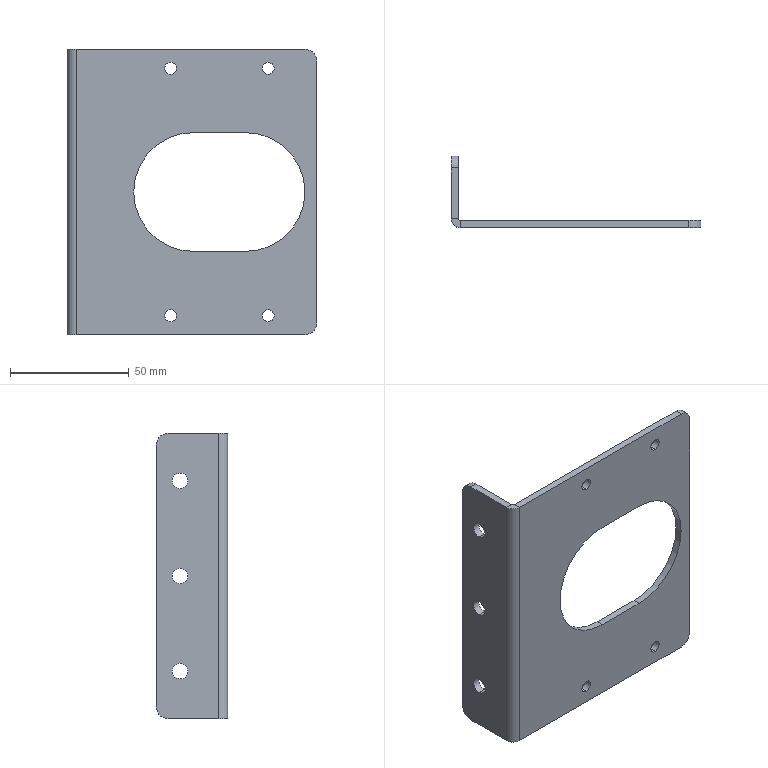Part | SolidWorks | features HoleWzd 2, BreakCorner 1, Cut 1, Extrusion 1, FlatPattern 1, ICE 1, SheetMetal 1, SolidToSheetMetal 1 | 1 solid | 36 faces | box 105 x 30 x 120 mm | volume 37376 mm3 | cylinder 22 | plane 14 | commonest cylinder face diameters 5 x8 6.6 x6 10 x4 50 x2 1.473 x1 7.473 x1
STEP:
#1=CARTESIAN_POINT('',(-52.5,5.,3.3));
#2=VERTEX_POINT('',#1);
#3=CARTESIAN_POINT('',(-52.5,5.,-3.3));
#4=VERTEX_POINT('',#3);
#5=CARTESIAN_POINT('',(-52.5,5.,0.));
#6=DIRECTION('',(1.,0.,0.));
#7=DIRECTION('',(0.,0.,-1.));
#8=AXIS2_PLACEMENT_3D('',#5,#6,#7);
#9=CIRCLE('',#8,3.3);
#10=EDGE_CURVE('',#2,#4,#9,.T.);
#11=ORIENTED_EDGE('',*,*,#10,.F.);
#12=CARTESIAN_POINT('',(-49.5,5.,3.3));
#13=VERTEX_POINT('',#12);
#14=CARTESIAN_POINT('',(-49.5,5.,3.3));
#15=DIRECTION('',(1.,0.,0.));
#16=VECTOR('',#15,1000.);
#17=LINE('',#14,#16);
#18=EDGE_CURVE('',#2,#13,#17,.T.);
#19=ORIENTED_EDGE('',*,*,#18,.T.);
#20=CARTESIAN_POINT('',(-49.5,5.,-3.3));
#21=VERTEX_POINT('',#20);
#22=CARTESIAN_POINT('',(-49.5,5.,0.));
#23=DIRECTION('',(1.,0.,0.));
#24=DIRECTION('',(0.,0.,-1.));
#25=AXIS2_PLACEMENT_3D('',#22,#23,#24);
#26=CIRCLE('',#25,3.3);
#27=EDGE_CURVE('',#13,#21,#26,.T.);
#28=ORIENTED_EDGE('',*,*,#27,.T.);
#29=CARTESIAN_POINT('',(-49.5,5.,-3.3));
#30=DIRECTION('',(1.,0.,0.));
#31=VECTOR('',#30,1000.);
#32=LINE('',#29,#31);
#33=EDGE_CURVE('',#4,#21,#32,.T.);
#34=ORIENTED_EDGE('',*,*,#33,.F.);
#35=EDGE_LOOP('',(#11,#19,#28,#34));
#36=FACE_OUTER_BOUND('',#35,.T.);
#37=CARTESIAN_POINT('',(-49.5,5.,0.));
#38=DIRECTION('',(1.,0.,0.));
#39=DIRECTION('',(0.,0.,-1.));
#40=AXIS2_PLACEMENT_3D('',#37,#38,#39);
#41=CYLINDRICAL_SURFACE('',#40,3.3);
#42=ADVANCED_FACE('',(#36),#41,.F.);
#43=CARTESIAN_POINT('',(-52.5,5.,43.3));
#44=VERTEX_POINT('',#43);
#45=CARTESIAN_POINT('',(-52.5,5.,36.7));
#46=VERTEX_POINT('',#45);
#47=CARTESIAN_POINT('',(-52.5,5.,40.));
#48=DIRECTION('',(1.,0.,0.));
#49=DIRECTION('',(0.,0.,-1.));
#50=AXIS2_PLACEMENT_3D('',#47,#48,#49);
#51=CIRCLE('',#50,3.3);
#52=EDGE_CURVE('',#44,#46,#51,.T.);
#53=ORIENTED_EDGE('',*,*,#52,.F.);
#54=CARTESIAN_POINT('',(-49.5,5.,43.3));
#55=VERTEX_POINT('',#54);
#56=CARTESIAN_POINT('',(-49.5,5.,43.3));
#57=DIRECTION('',(1.,0.,0.));
#58=VECTOR('',#57,1000.);
#59=LINE('',#56,#58);
#60=EDGE_CURVE('',#44,#55,#59,.T.);
#61=ORIENTED_EDGE('',*,*,#60,.T.);
#62=CARTESIAN_POINT('',(-49.5,5.,36.7));
#63=VERTEX_POINT('',#62);
#64=CARTESIAN_POINT('',(-49.5,5.,40.));
#65=DIRECTION('',(1.,0.,0.));
#66=DIRECTION('',(0.,0.,-1.));
#67=AXIS2_PLACEMENT_3D('',#64,#65,#66);
#68=CIRCLE('',#67,3.3);
#69=EDGE_CURVE('',#55,#63,#68,.T.);
#70=ORIENTED_EDGE('',*,*,#69,.T.);
#71=CARTESIAN_POINT('',(-49.5,5.,36.7));
#72=DIRECTION('',(1.,0.,0.));
#73=VECTOR('',#72,1000.);
#74=LINE('',#71,#73);
#75=EDGE_CURVE('',#46,#63,#74,.T.);
#76=ORIENTED_EDGE('',*,*,#75,.F.);
#77=EDGE_LOOP('',(#53,#61,#70,#76));
#78=FACE_OUTER_BOUND('',#77,.T.);
#79=CARTESIAN_POINT('',(-49.5,5.,40.));
#80=DIRECTION('',(1.,0.,0.));
#81=DIRECTION('',(0.,0.,-1.));
#82=AXIS2_PLACEMENT_3D('',#79,#80,#81);
#83=CYLINDRICAL_SURFACE('',#82,3.3);
#84=ADVANCED_FACE('',(#78),#83,.F.);
#85=CARTESIAN_POINT('',(-52.5,5.,-36.7));
#86=VERTEX_POINT('',#85);
#87=CARTESIAN_POINT('',(-52.5,5.,-43.3));
#88=VERTEX_POINT('',#87);
#89=CARTESIAN_POINT('',(-52.5,5.,-40.));
#90=DIRECTION('',(1.,0.,0.));
#91=DIRECTION('',(0.,0.,-1.));
#92=AXIS2_PLACEMENT_3D('',#89,#90,#91);
#93=CIRCLE('',#92,3.3);
#94=EDGE_CURVE('',#86,#88,#93,.T.);
#95=ORIENTED_EDGE('',*,*,#94,.F.);
#96=CARTESIAN_POINT('',(-49.5,5.,-36.7));
#97=VERTEX_POINT('',#96);
#98=CARTESIAN_POINT('',(-49.5,5.,-36.7));
#99=DIRECTION('',(1.,0.,0.));
#100=VECTOR('',#99,1000.);
#101=LINE('',#98,#100);
#102=EDGE_CURVE('',#86,#97,#101,.T.);
#103=ORIENTED_EDGE('',*,*,#102,.T.);
#104=CARTESIAN_POINT('',(-49.5,5.,-43.3));
#105=VERTEX_POINT('',#104);
#106=CARTESIAN_POINT('',(-49.5,5.,-40.));
#107=DIRECTION('',(1.,0.,0.));
#108=DIRECTION('',(0.,0.,-1.));
#109=AXIS2_PLACEMENT_3D('',#106,#107,#108);
#110=CIRCLE('',#109,3.3);
#111=EDGE_CURVE('',#97,#105,#110,.T.);
#112=ORIENTED_EDGE('',*,*,#111,.T.);
#113=CARTESIAN_POINT('',(-49.5,5.,-43.3));
#114=DIRECTION('',(1.,0.,0.));
#115=VECTOR('',#114,1000.);
#116=LINE('',#113,#115);
#117=EDGE_CURVE('',#88,#105,#116,.T.);
#118=ORIENTED_EDGE('',*,*,#117,.F.);
#119=EDGE_LOOP('',(#95,#103,#112,#118));
#120=FACE_OUTER_BOUND('',#119,.T.);
#121=CARTESIAN_POINT('',(-49.5,5.,-40.));
#122=DIRECTION('',(1.,0.,0.));
#123=DIRECTION('',(0.,0.,-1.));
#124=AXIS2_PLACEMENT_3D('',#121,#122,#123);
#125=CYLINDRICAL_SURFACE('',#124,3.3);
#126=ADVANCED_FACE('',(#120),#125,.F.);
#127=CARTESIAN_POINT('',(-9.,-15.,-54.5));
#128=VERTEX_POINT('',#127);
#129=CARTESIAN_POINT('',(-9.,-15.,-49.5));
#130=VERTEX_POINT('',#129);
#131=CARTESIAN_POINT('',(-9.,-15.,-52.));
#132=DIRECTION('',(0.,1.,0.));
#133=DIRECTION('',(0.,0.,1.));
#134=AXIS2_PLACEMENT_3D('',#131,#132,#133);
#135=CIRCLE('',#134,2.5);
#136=EDGE_CURVE('',#128,#130,#135,.T.);
#137=ORIENTED_EDGE('',*,*,#136,.F.);
#138=CARTESIAN_POINT('',(-9.,-12.,-54.5));
#139=VERTEX_POINT('',#138);
#140=CARTESIAN_POINT('',(-9.,-12.,-54.5));
#141=DIRECTION('',(0.,1.,0.));
#142=VECTOR('',#141,1000.);
#143=LINE('',#140,#142);
#144=EDGE_CURVE('',#128,#139,#143,.T.);
#145=ORIENTED_EDGE('',*,*,#144,.T.);
#146=CARTESIAN_POINT('',(-9.,-12.,-49.5));
#147=VERTEX_POINT('',#146);
#148=CARTESIAN_POINT('',(-9.,-12.,-52.));
#149=DIRECTION('',(0.,1.,0.));
#150=DIRECTION('',(0.,0.,1.));
#151=AXIS2_PLACEMENT_3D('',#148,#149,#150);
#152=CIRCLE('',#151,2.5);
#153=EDGE_CURVE('',#139,#147,#152,.T.);
#154=ORIENTED_EDGE('',*,*,#153,.T.);
#155=CARTESIAN_POINT('',(-9.,-12.,-49.5));
#156=DIRECTION('',(0.,1.,0.));
#157=VECTOR('',#156,1000.);
#158=LINE('',#155,#157);
#159=EDGE_CURVE('',#130,#147,#158,.T.);
#160=ORIENTED_EDGE('',*,*,#159,.F.);
#161=EDGE_LOOP('',(#137,#145,#154,#160));
#162=FACE_OUTER_BOUND('',#161,.T.);
#163=CARTESIAN_POINT('',(-9.,-12.,-52.));
#164=DIRECTION('',(0.,1.,0.));
#165=DIRECTION('',(0.,0.,1.));
#166=AXIS2_PLACEMENT_3D('',#163,#164,#165);
#167=CYLINDRICAL_SURFACE('',#166,2.5);
#168=ADVANCED_FACE('',(#162),#167,.F.);
#169=CARTESIAN_POINT('',(32.,-15.,-54.5));
#170=VERTEX_POINT('',#169);
#171=CARTESIAN_POINT('',(32.,-15.,-49.5));
#172=VERTEX_POINT('',#171);
#173=CARTESIAN_POINT('',(32.,-15.,-52.));
#174=DIRECTION('',(0.,1.,0.));
#175=DIRECTION('',(0.,0.,1.));
#176=AXIS2_PLACEMENT_3D('',#173,#174,#175);
#177=CIRCLE('',#176,2.5);
#178=EDGE_CURVE('',#170,#172,#177,.T.);
#179=ORIENTED_EDGE('',*,*,#178,.F.);
#180=CARTESIAN_POINT('',(32.,-12.,-54.5));
#181=VERTEX_POINT('',#180);
#182=CARTESIAN_POINT('',(32.,-12.,-54.5));
#183=DIRECTION('',(0.,1.,0.));
#184=VECTOR('',#183,1000.);
#185=LINE('',#182,#184);
#186=EDGE_CURVE('',#170,#181,#185,.T.);
#187=ORIENTED_EDGE('',*,*,#186,.T.);
#188=CARTESIAN_POINT('',(32.,-12.,-49.5));
#189=VERTEX_POINT('',#188);
#190=CARTESIAN_POINT('',(32.,-12.,-52.));
#191=DIRECTION('',(0.,1.,0.));
#192=DIRECTION('',(0.,0.,1.));
#193=AXIS2_PLACEMENT_3D('',#190,#191,#192);
#194=CIRCLE('',#193,2.5);
#195=EDGE_CURVE('',#181,#189,#194,.T.);
#196=ORIENTED_EDGE('',*,*,#195,.T.);
#197=CARTESIAN_POINT('',(32.,-12.,-49.5));
#198=DIRECTION('',(0.,1.,0.));
#199=VECTOR('',#198,1000.);
#200=LINE('',#197,#199);
#201=EDGE_CURVE('',#172,#189,#200,.T.);
#202=ORIENTED_EDGE('',*,*,#201,.F.);
#203=EDGE_LOOP('',(#179,#187,#196,#202));
#204=FACE_OUTER_BOUND('',#203,.T.);
#205=CARTESIAN_POINT('',(32.,-12.,-52.));
#206=DIRECTION('',(0.,1.,0.));
#207=DIRECTION('',(0.,0.,1.));
#208=AXIS2_PLACEMENT_3D('',#205,#206,#207);
#209=CYLINDRICAL_SURFACE('',#208,2.5);
#210=ADVANCED_FACE('',(#204),#209,.F.);
#211=CARTESIAN_POINT('',(32.,-15.,49.5));
#212=VERTEX_POINT('',#211);
#213=CARTESIAN_POINT('',(32.,-15.,54.5));
#214=VERTEX_POINT('',#213);
#215=CARTESIAN_POINT('',(32.,-15.,52.));
#216=DIRECTION('',(0.,1.,0.));
#217=DIRECTION('',(0.,0.,1.));
#218=AXIS2_PLACEMENT_3D('',#215,#216,#217);
#219=CIRCLE('',#218,2.5);
#220=EDGE_CURVE('',#212,#214,#219,.T.);
#221=ORIENTED_EDGE('',*,*,#220,.F.);
#222=CARTESIAN_POINT('',(32.,-12.,49.5));
#223=VERTEX_POINT('',#222);
#224=CARTESIAN_POINT('',(32.,-12.,49.5));
#225=DIRECTION('',(0.,1.,0.));
#226=VECTOR('',#225,1000.);
#227=LINE('',#224,#226);
#228=EDGE_CURVE('',#212,#223,#227,.T.);
#229=ORIENTED_EDGE('',*,*,#228,.T.);
#230=CARTESIAN_POINT('',(32.,-12.,54.5));
#231=VERTEX_POINT('',#230);
#232=CARTESIAN_POINT('',(32.,-12.,52.));
#233=DIRECTION('',(0.,1.,0.));
#234=DIRECTION('',(0.,0.,1.));
#235=AXIS2_PLACEMENT_3D('',#232,#233,#234);
#236=CIRCLE('',#235,2.5);
#237=EDGE_CURVE('',#223,#231,#236,.T.);
#238=ORIENTED_EDGE('',*,*,#237,.T.);
#239=CARTESIAN_POINT('',(32.,-12.,54.5));
#240=DIRECTION('',(0.,1.,0.));
#241=VECTOR('',#240,1000.);
#242=LINE('',#239,#241);
#243=EDGE_CURVE('',#214,#231,#242,.T.);
#244=ORIENTED_EDGE('',*,*,#243,.F.);
#245=EDGE_LOOP('',(#221,#229,#238,#244));
#246=FACE_OUTER_BOUND('',#245,.T.);
#247=CARTESIAN_POINT('',(32.,-12.,52.));
#248=DIRECTION('',(0.,1.,0.));
#249=DIRECTION('',(0.,0.,1.));
#250=AXIS2_PLACEMENT_3D('',#247,#248,#249);
#251=CYLINDRICAL_SURFACE('',#250,2.5);
#252=ADVANCED_FACE('',(#246),#251,.F.);
#253=CARTESIAN_POINT('',(-9.,-15.,49.5));
#254=VERTEX_POINT('',#253);
#255=CARTESIAN_POINT('',(-9.,-15.,54.5));
#256=VERTEX_POINT('',#255);
#257=CARTESIAN_POINT('',(-9.,-15.,52.));
#258=DIRECTION('',(0.,1.,0.));
#259=DIRECTION('',(0.,0.,1.));
#260=AXIS2_PLACEMENT_3D('',#257,#258,#259);
#261=CIRCLE('',#260,2.5);
#262=EDGE_CURVE('',#254,#256,#261,.T.);
#263=ORIENTED_EDGE('',*,*,#262,.F.);
#264=CARTESIAN_POINT('',(-9.,-12.,49.5));
#265=VERTEX_POINT('',#264);
#266=CARTESIAN_POINT('',(-9.,-12.,49.5));
#267=DIRECTION('',(0.,1.,0.));
#268=VECTOR('',#267,1000.);
#269=LINE('',#266,#268);
#270=EDGE_CURVE('',#254,#265,#269,.T.);
#271=ORIENTED_EDGE('',*,*,#270,.T.);
#272=CARTESIAN_POINT('',(-9.,-12.,54.5));
#273=VERTEX_POINT('',#272);
#274=CARTESIAN_POINT('',(-9.,-12.,52.));
#275=DIRECTION('',(0.,1.,0.));
#276=DIRECTION('',(0.,0.,1.));
#277=AXIS2_PLACEMENT_3D('',#274,#275,#276);
#278=CIRCLE('',#277,2.5);
#279=EDGE_CURVE('',#265,#273,#278,.T.);
#280=ORIENTED_EDGE('',*,*,#279,.T.);
#281=CARTESIAN_POINT('',(-9.,-12.,54.5));
#282=DIRECTION('',(0.,1.,0.));
#283=VECTOR('',#282,1000.);
#284=LINE('',#281,#283);
#285=EDGE_CURVE('',#256,#273,#284,.T.);
#286=ORIENTED_EDGE('',*,*,#285,.F.);
#287=EDGE_LOOP('',(#263,#271,#280,#286));
#288=FACE_OUTER_BOUND('',#287,.T.);
#289=CARTESIAN_POINT('',(-9.,-12.,52.));
#290=DIRECTION('',(0.,1.,0.));
#291=DIRECTION('',(0.,0.,1.));
#292=AXIS2_PLACEMENT_3D('',#289,#290,#291);
#293=CYLINDRICAL_SURFACE('',#292,2.5);
#294=ADVANCED_FACE('',(#288),#293,.F.);
#295=CARTESIAN_POINT('',(-48.763,-12.,-60.));
#296=VERTEX_POINT('',#295);
#297=CARTESIAN_POINT('',(47.5,-12.,-60.));
#298=VERTEX_POINT('',#297);
#299=CARTESIAN_POINT('',(-52.5,-12.,-60.));
#300=DIRECTION('',(1.,0.,0.));
#301=VECTOR('',#300,1000.);
#302=LINE('',#299,#301);
#303=EDGE_CURVE('',#296,#298,#302,.T.);
#304=ORIENTED_EDGE('',*,*,#303,.T.);
#305=CARTESIAN_POINT('',(47.5,-15.,-60.));
#306=VERTEX_POINT('',#305);
#307=CARTESIAN_POINT('',(47.5,-15.,-60.));
#308=DIRECTION('',(0.,-1.,0.));
#309=VECTOR('',#308,1000.);
#310=LINE('',#307,#309);
#311=EDGE_CURVE('',#298,#306,#310,.T.);
#312=ORIENTED_EDGE('',*,*,#311,.T.);
#313=CARTESIAN_POINT('',(-48.763,-15.,-60.));
#314=VERTEX_POINT('',#313);
#315=CARTESIAN_POINT('',(-52.5,-15.,-60.));
#316=DIRECTION('',(1.,0.,0.));
#317=VECTOR('',#316,1000.);
#318=LINE('',#315,#317);
#319=EDGE_CURVE('',#314,#306,#318,.T.);
#320=ORIENTED_EDGE('',*,*,#319,.F.);
#321=CARTESIAN_POINT('',(-48.763,-15.,-60.));
#322=DIRECTION('',(0.,-1.,0.));
#323=VECTOR('',#322,1000.);
#324=LINE('',#321,#323);
#325=EDGE_CURVE('',#296,#314,#324,.T.);
#326=ORIENTED_EDGE('',*,*,#325,.F.);
#327=EDGE_LOOP('',(#304,#312,#320,#326));
#328=FACE_OUTER_BOUND('',#327,.T.);
#329=CARTESIAN_POINT('',(-52.5,-15.,-60.));
#330=DIRECTION('',(0.,0.,1.));
#331=DIRECTION('',(1.,0.,0.));
#332=AXIS2_PLACEMENT_3D('',#329,#330,#331);
#333=PLANE('',#332);
#334=ADVANCED_FACE('',(#328),#333,.F.);
#335=CARTESIAN_POINT('',(52.5,-15.,55.));
#336=VERTEX_POINT('',#335);
#337=CARTESIAN_POINT('',(52.5,-15.,-55.));
#338=VERTEX_POINT('',#337);
#339=CARTESIAN_POINT('',(52.5,-15.,60.));
#340=DIRECTION('',(0.,0.,-1.));
#341=VECTOR('',#340,1000.);
#342=LINE('',#339,#341);
#343=EDGE_CURVE('',#336,#338,#342,.T.);
#344=ORIENTED_EDGE('',*,*,#343,.T.);
#345=CARTESIAN_POINT('',(52.5,-12.,-55.));
#346=VERTEX_POINT('',#345);
#347=CARTESIAN_POINT('',(52.5,-15.,-55.));
#348=DIRECTION('',(0.,1.,0.));
#349=VECTOR('',#348,1000.);
#350=LINE('',#347,#349);
#351=EDGE_CURVE('',#338,#346,#350,.T.);
#352=ORIENTED_EDGE('',*,*,#351,.T.);
#353=CARTESIAN_POINT('',(52.5,-12.,55.));
#354=VERTEX_POINT('',#353);
#355=CARTESIAN_POINT('',(52.5,-12.,60.));
#356=DIRECTION('',(0.,0.,-1.));
#357=VECTOR('',#356,1000.);
#358=LINE('',#355,#357);
#359=EDGE_CURVE('',#354,#346,#358,.T.);
#360=ORIENTED_EDGE('',*,*,#359,.F.);
#361=CARTESIAN_POINT('',(52.5,-15.,55.));
#362=DIRECTION('',(0.,-1.,0.));
#363=VECTOR('',#362,1000.);
#364=LINE('',#361,#363);
#365=EDGE_CURVE('',#354,#336,#364,.T.);
#366=ORIENTED_EDGE('',*,*,#365,.T.);
#367=EDGE_LOOP('',(#344,#352,#360,#366));
#368=FACE_OUTER_BOUND('',#367,.T.);
#369=CARTESIAN_POINT('',(52.5,-15.,60.));
#370=DIRECTION('',(1.,0.,0.));
#371=DIRECTION('',(0.,0.,-1.));
#372=AXIS2_PLACEMENT_3D('',#369,#370,#371);
#373=PLANE('',#372);
#374=ADVANCED_FACE('',(#368),#373,.T.);
#375=CARTESIAN_POINT('',(-48.763,-15.,60.));
#376=VERTEX_POINT('',#375);
#377=CARTESIAN_POINT('',(47.5,-15.,60.));
#378=VERTEX_POINT('',#377);
#379=CARTESIAN_POINT('',(-52.5,-15.,60.));
#380=DIRECTION('',(1.,0.,0.));
#381=VECTOR('',#380,1000.);
#382=LINE('',#379,#381);
#383=EDGE_CURVE('',#376,#378,#382,.T.);
#384=ORIENTED_EDGE('',*,*,#383,.T.);
#385=CARTESIAN_POINT('',(47.5,-12.,60.));
#386=VERTEX_POINT('',#385);
#387=CARTESIAN_POINT('',(47.5,-15.,60.));
#388=DIRECTION('',(0.,1.,0.));
#389=VECTOR('',#388,1000.);
#390=LINE('',#387,#389);
#391=EDGE_CURVE('',#378,#386,#390,.T.);
#392=ORIENTED_EDGE('',*,*,#391,.T.);
#393=CARTESIAN_POINT('',(-48.763,-12.,60.));
#394=VERTEX_POINT('',#393);
#395=CARTESIAN_POINT('',(-52.5,-12.,60.));
#396=DIRECTION('',(1.,0.,0.));
#397=VECTOR('',#396,1000.);
#398=LINE('',#395,#397);
#399=EDGE_CURVE('',#394,#386,#398,.T.);
#400=ORIENTED_EDGE('',*,*,#399,.F.);
#401=CARTESIAN_POINT('',(-48.763,-15.,60.));
#402=DIRECTION('',(0.,-1.,0.));
#403=VECTOR('',#402,1000.);
#404=LINE('',#401,#403);
#405=EDGE_CURVE('',#394,#376,#404,.T.);
#406=ORIENTED_EDGE('',*,*,#405,.T.);
#407=EDGE_LOOP('',(#384,#392,#400,#406));
#408=FACE_OUTER_BOUND('',#407,.T.);
#409=CARTESIAN_POINT('',(-52.5,-15.,60.));
#410=DIRECTION('',(0.,0.,1.));
#411=DIRECTION('',(1.,0.,0.));
#412=AXIS2_PLACEMENT_3D('',#409,#410,#411);
#413=PLANE('',#412);
#414=ADVANCED_FACE('',(#408),#413,.T.);
#415=ORIENTED_EDGE('',*,*,#405,.F.);
#416=CARTESIAN_POINT('',(-49.5,-11.263,60.));
#417=VERTEX_POINT('',#416);
#418=CARTESIAN_POINT('',(-48.763,-11.263,60.));
#419=DIRECTION('',(0.,0.,-1.));
#420=DIRECTION('',(-1.,0.,0.));
#421=AXIS2_PLACEMENT_3D('',#418,#419,#420);
#422=CIRCLE('',#421,0.7366);
#423=EDGE_CURVE('',#394,#417,#422,.T.);
#424=ORIENTED_EDGE('',*,*,#423,.T.);
#425=CARTESIAN_POINT('',(-52.5,-11.263,60.));
#426=VERTEX_POINT('',#425);
#427=CARTESIAN_POINT('',(-52.5,-11.263,60.));
#428=DIRECTION('',(-1.,0.,0.));
#429=VECTOR('',#428,1000.);
#430=LINE('',#427,#429);
#431=EDGE_CURVE('',#417,#426,#430,.T.);
#432=ORIENTED_EDGE('',*,*,#431,.T.);
#433=CARTESIAN_POINT('',(-48.763,-11.263,60.));
#434=DIRECTION('',(0.,0.,-1.));
#435=DIRECTION('',(1.,0.,0.));
#436=AXIS2_PLACEMENT_3D('',#433,#434,#435);
#437=CIRCLE('',#436,3.737);
#438=EDGE_CURVE('',#376,#426,#437,.T.);
#439=ORIENTED_EDGE('',*,*,#438,.F.);
#440=EDGE_LOOP('',(#415,#424,#432,#439));
#441=FACE_OUTER_BOUND('',#440,.T.);
#442=CARTESIAN_POINT('',(-48.763,-11.263,60.));
#443=DIRECTION('',(0.,0.,-1.));
#444=DIRECTION('',(-1.,0.,0.));
#445=AXIS2_PLACEMENT_3D('',#442,#443,#444);
#446=PLANE('',#445);
#447=ADVANCED_FACE('',(#441),#446,.F.);
#448=CARTESIAN_POINT('',(-49.5,10.,60.));
#449=VERTEX_POINT('',#448);
#450=CARTESIAN_POINT('',(-49.5,-15.,60.));
#451=DIRECTION('',(0.,-1.,0.));
#452=VECTOR('',#451,1000.);
#453=LINE('',#450,#452);
#454=EDGE_CURVE('',#449,#417,#453,.T.);
#455=ORIENTED_EDGE('',*,*,#454,.F.);
#456=CARTESIAN_POINT('',(-52.5,10.,60.));
#457=VERTEX_POINT('',#456);
#458=CARTESIAN_POINT('',(-52.5,10.,60.));
#459=DIRECTION('',(-1.,0.,0.));
#460=VECTOR('',#459,1000.);
#461=LINE('',#458,#460);
#462=EDGE_CURVE('',#449,#457,#461,.T.);
#463=ORIENTED_EDGE('',*,*,#462,.T.);
#464=CARTESIAN_POINT('',(-52.5,-15.,60.));
#465=DIRECTION('',(0.,-1.,0.));
#466=VECTOR('',#465,1000.);
#467=LINE('',#464,#466);
#468=EDGE_CURVE('',#457,#426,#467,.T.);
#469=ORIENTED_EDGE('',*,*,#468,.T.);
#470=ORIENTED_EDGE('',*,*,#431,.F.);
#471=EDGE_LOOP('',(#455,#463,#469,#470));
#472=FACE_OUTER_BOUND('',#471,.T.);
#473=CARTESIAN_POINT('',(-52.5,-15.,60.));
#474=DIRECTION('',(0.,0.,1.));
#475=DIRECTION('',(0.,-1.,0.));
#476=AXIS2_PLACEMENT_3D('',#473,#474,#475);
#477=PLANE('',#476);
#478=ADVANCED_FACE('',(#472),#477,.T.);
#479=CARTESIAN_POINT('',(-52.5,15.,55.));
#480=VERTEX_POINT('',#479);
#481=CARTESIAN_POINT('',(-52.5,15.,-55.));
#482=VERTEX_POINT('',#481);
#483=CARTESIAN_POINT('',(-52.5,15.,60.));
#484=DIRECTION('',(0.,0.,-1.));
#485=VECTOR('',#484,1000.);
#486=LINE('',#483,#485);
#487=EDGE_CURVE('',#480,#482,#486,.T.);
#488=ORIENTED_EDGE('',*,*,#487,.F.);
#489=CARTESIAN_POINT('',(-49.5,15.,55.));
#490=VERTEX_POINT('',#489);
#491=CARTESIAN_POINT('',(-52.5,15.,55.));
#492=DIRECTION('',(1.,0.,0.));
#493=VECTOR('',#492,1000.);
#494=LINE('',#491,#493);
#495=EDGE_CURVE('',#480,#490,#494,.T.);
#496=ORIENTED_EDGE('',*,*,#495,.T.);
#497=CARTESIAN_POINT('',(-49.5,15.,-55.));
#498=VERTEX_POINT('',#497);
#499=CARTESIAN_POINT('',(-49.5,15.,60.));
#500=DIRECTION('',(0.,0.,-1.));
#501=VECTOR('',#500,1000.);
#502=LINE('',#499,#501);
#503=EDGE_CURVE('',#490,#498,#502,.T.);
#504=ORIENTED_EDGE('',*,*,#503,.T.);
#505=CARTESIAN_POINT('',(-52.5,15.,-55.));
#506=DIRECTION('',(-1.,0.,0.));
#507=VECTOR('',#506,1000.);
#508=LINE('',#505,#507);
#509=EDGE_CURVE('',#498,#482,#508,.T.);
#510=ORIENTED_EDGE('',*,*,#509,.T.);
#511=EDGE_LOOP('',(#488,#496,#504,#510));
#512=FACE_OUTER_BOUND('',#511,.T.);
#513=CARTESIAN_POINT('',(-52.5,15.,60.));
#514=DIRECTION('',(0.,-1.,0.));
#515=DIRECTION('',(0.,0.,-1.));
#516=AXIS2_PLACEMENT_3D('',#513,#514,#515);
#517=PLANE('',#516);
#518=ADVANCED_FACE('',(#512),#517,.F.);
#519=CARTESIAN_POINT('',(-52.5,10.,-60.));
#520=VERTEX_POINT('',#519);
#521=CARTESIAN_POINT('',(-52.5,-11.263,-60.));
#522=VERTEX_POINT('',#521);
#523=CARTESIAN_POINT('',(-52.5,-15.,-60.));
#524=DIRECTION('',(0.,-1.,0.));
#525=VECTOR('',#524,1000.);
#526=LINE('',#523,#525);
#527=EDGE_CURVE('',#520,#522,#526,.T.);
#528=ORIENTED_EDGE('',*,*,#527,.F.);
#529=CARTESIAN_POINT('',(-49.5,10.,-60.));
#530=VERTEX_POINT('',#529);
#531=CARTESIAN_POINT('',(-52.5,10.,-60.));
#532=DIRECTION('',(1.,0.,0.));
#533=VECTOR('',#532,1000.);
#534=LINE('',#531,#533);
#535=EDGE_CURVE('',#520,#530,#534,.T.);
#536=ORIENTED_EDGE('',*,*,#535,.T.);
#537=CARTESIAN_POINT('',(-49.5,-11.263,-60.));
#538=VERTEX_POINT('',#537);
#539=CARTESIAN_POINT('',(-49.5,-15.,-60.));
#540=DIRECTION('',(0.,-1.,0.));
#541=VECTOR('',#540,1000.);
#542=LINE('',#539,#541);
#543=EDGE_CURVE('',#530,#538,#542,.T.);
#544=ORIENTED_EDGE('',*,*,#543,.T.);
#545=CARTESIAN_POINT('',(-52.5,-11.263,-60.));
#546=DIRECTION('',(-1.,0.,0.));
#547=VECTOR('',#546,1000.);
#548=LINE('',#545,#547);
#549=EDGE_CURVE('',#538,#522,#548,.T.);
#550=ORIENTED_EDGE('',*,*,#549,.T.);
#551=EDGE_LOOP('',(#528,#536,#544,#550));
#552=FACE_OUTER_BOUND('',#551,.T.);
#553=CARTESIAN_POINT('',(-52.5,-15.,-60.));
#554=DIRECTION('',(0.,0.,1.));
#555=DIRECTION('',(0.,-1.,0.));
#556=AXIS2_PLACEMENT_3D('',#553,#554,#555);
#557=PLANE('',#556);
#558=ADVANCED_FACE('',(#552),#557,.F.);
#559=CARTESIAN_POINT('',(-48.763,-11.263,-60.));
#560=DIRECTION('',(0.,0.,1.));
#561=DIRECTION('',(-1.,0.,0.));
#562=AXIS2_PLACEMENT_3D('',#559,#560,#561);
#563=CIRCLE('',#562,0.7366);
#564=EDGE_CURVE('',#538,#296,#563,.T.);
#565=ORIENTED_EDGE('',*,*,#564,.T.);
#566=ORIENTED_EDGE('',*,*,#325,.T.);
#567=CARTESIAN_POINT('',(-48.763,-11.263,-60.));
#568=DIRECTION('',(0.,0.,1.));
#569=DIRECTION('',(-1.,0.,0.));
#570=AXIS2_PLACEMENT_3D('',#567,#568,#569);
#571=CIRCLE('',#570,3.737);
#572=EDGE_CURVE('',#522,#314,#571,.T.);
#573=ORIENTED_EDGE('',*,*,#572,.F.);
#574=ORIENTED_EDGE('',*,*,#549,.F.);
#575=EDGE_LOOP('',(#565,#566,#573,#574));
#576=FACE_OUTER_BOUND('',#575,.T.);
#577=CARTESIAN_POINT('',(-48.763,-11.263,-60.));
#578=DIRECTION('',(0.,0.,1.));
#579=DIRECTION('',(1.,0.,0.));
#580=AXIS2_PLACEMENT_3D('',#577,#578,#579);
#581=PLANE('',#580);
#582=ADVANCED_FACE('',(#576),#581,.F.);
#583=CARTESIAN_POINT('',(-52.5,5.,0.));
#584=DIRECTION('',(1.,0.,0.));
#585=DIRECTION('',(0.,0.,-1.));
#586=AXIS2_PLACEMENT_3D('',#583,#584,#585);
#587=CIRCLE('',#586,3.3);
#588=EDGE_CURVE('',#4,#2,#587,.T.);
#589=ORIENTED_EDGE('',*,*,#588,.T.);
#590=ORIENTED_EDGE('',*,*,#10,.T.);
#591=EDGE_LOOP('',(#589,#590));
#592=FACE_BOUND('',#591,.T.);
#593=CARTESIAN_POINT('',(-52.5,5.,40.));
#594=DIRECTION('',(1.,0.,0.));
#595=DIRECTION('',(0.,0.,-1.));
#596=AXIS2_PLACEMENT_3D('',#593,#594,#595);
#597=CIRCLE('',#596,3.3);
#598=EDGE_CURVE('',#46,#44,#597,.T.);
#599=ORIENTED_EDGE('',*,*,#598,.T.);
#600=ORIENTED_EDGE('',*,*,#52,.T.);
#601=EDGE_LOOP('',(#599,#600));
#602=FACE_BOUND('',#601,.T.);
#603=CARTESIAN_POINT('',(-52.5,5.,-40.));
#604=DIRECTION('',(1.,0.,0.));
#605=DIRECTION('',(0.,0.,-1.));
#606=AXIS2_PLACEMENT_3D('',#603,#604,#605);
#607=CIRCLE('',#606,3.3);
#608=EDGE_CURVE('',#88,#86,#607,.T.);
#609=ORIENTED_EDGE('',*,*,#608,.T.);
#610=ORIENTED_EDGE('',*,*,#94,.T.);
#611=EDGE_LOOP('',(#609,#610));
#612=FACE_BOUND('',#611,.T.);
#613=ORIENTED_EDGE('',*,*,#468,.F.);
#614=CARTESIAN_POINT('',(-52.5,10.,55.));
#615=DIRECTION('',(-1.,0.,0.));
#616=DIRECTION('',(0.,0.,-1.));
#617=AXIS2_PLACEMENT_3D('',#614,#615,#616);
#618=CIRCLE('',#617,5.);
#619=EDGE_CURVE('',#457,#480,#618,.T.);
#620=ORIENTED_EDGE('',*,*,#619,.T.);
#621=ORIENTED_EDGE('',*,*,#487,.T.);
#622=CARTESIAN_POINT('',(-52.5,10.,-55.));
#623=DIRECTION('',(-1.,0.,0.));
#624=DIRECTION('',(0.,0.,-1.));
#625=AXIS2_PLACEMENT_3D('',#622,#623,#624);
#626=CIRCLE('',#625,5.);
#627=EDGE_CURVE('',#482,#520,#626,.T.);
#628=ORIENTED_EDGE('',*,*,#627,.T.);
#629=ORIENTED_EDGE('',*,*,#527,.T.);
#630=CARTESIAN_POINT('',(-52.5,-11.263,60.));
#631=DIRECTION('',(0.,0.,1.));
#632=VECTOR('',#631,1000.);
#633=LINE('',#630,#632);
#634=EDGE_CURVE('',#522,#426,#633,.T.);
#635=ORIENTED_EDGE('',*,*,#634,.T.);
#636=EDGE_LOOP('',(#613,#620,#621,#628,#629,#635));
#637=FACE_OUTER_BOUND('',#636,.T.);
#638=CARTESIAN_POINT('',(-52.5,-15.,60.));
#639=DIRECTION('',(1.,0.,0.));
#640=DIRECTION('',(0.,0.,-1.));
#641=AXIS2_PLACEMENT_3D('',#638,#639,#640);
#642=PLANE('',#641);
#643=ADVANCED_FACE('',(#592,#602,#612,#637),#642,.F.);
#644=CARTESIAN_POINT('',(-9.,-15.,-52.));
#645=DIRECTION('',(0.,1.,0.));
#646=DIRECTION('',(0.,0.,1.));
#647=AXIS2_PLACEMENT_3D('',#644,#645,#646);
#648=CIRCLE('',#647,2.5);
#649=EDGE_CURVE('',#130,#128,#648,.T.);
#650=ORIENTED_EDGE('',*,*,#649,.T.);
#651=ORIENTED_EDGE('',*,*,#136,.T.);
#652=EDGE_LOOP('',(#650,#651));
#653=FACE_BOUND('',#652,.T.);
#654=CARTESIAN_POINT('',(32.,-15.,-52.));
#655=DIRECTION('',(0.,1.,0.));
#656=DIRECTION('',(0.,0.,1.));
#657=AXIS2_PLACEMENT_3D('',#654,#655,#656);
#658=CIRCLE('',#657,2.5);
#659=EDGE_CURVE('',#172,#170,#658,.T.);
#660=ORIENTED_EDGE('',*,*,#659,.T.);
#661=ORIENTED_EDGE('',*,*,#178,.T.);
#662=EDGE_LOOP('',(#660,#661));
#663=FACE_BOUND('',#662,.T.);
#664=CARTESIAN_POINT('',(32.,-15.,52.));
#665=DIRECTION('',(0.,1.,0.));
#666=DIRECTION('',(0.,0.,1.));
#667=AXIS2_PLACEMENT_3D('',#664,#665,#666);
#668=CIRCLE('',#667,2.5);
#669=EDGE_CURVE('',#214,#212,#668,.T.);
#670=ORIENTED_EDGE('',*,*,#669,.T.);
#671=ORIENTED_EDGE('',*,*,#220,.T.);
#672=EDGE_LOOP('',(#670,#671));
#673=FACE_BOUND('',#672,.T.);
#674=CARTESIAN_POINT('',(-9.,-15.,52.));
#675=DIRECTION('',(0.,1.,0.));
#676=DIRECTION('',(0.,0.,1.));
#677=AXIS2_PLACEMENT_3D('',#674,#675,#676);
#678=CIRCLE('',#677,2.5);
#679=EDGE_CURVE('',#256,#254,#678,.T.);
#680=ORIENTED_EDGE('',*,*,#679,.T.);
#681=ORIENTED_EDGE('',*,*,#262,.T.);
#682=EDGE_LOOP('',(#680,#681));
#683=FACE_BOUND('',#682,.T.);
#684=CARTESIAN_POINT('',(22.5,-15.,25.));
#685=VERTEX_POINT('',#684);
#686=CARTESIAN_POINT('',(0.5,-15.,25.));
#687=VERTEX_POINT('',#686);
#688=CARTESIAN_POINT('',(22.5,-15.,25.));
#689=DIRECTION('',(-1.,0.,0.));
#690=VECTOR('',#689,1000.);
#691=LINE('',#688,#690);
#692=EDGE_CURVE('',#685,#687,#691,.T.);
#693=ORIENTED_EDGE('',*,*,#692,.F.);
#694=CARTESIAN_POINT('',(22.5,-15.,-25.));
#695=VERTEX_POINT('',#694);
#696=CARTESIAN_POINT('',(22.5,-15.,0.));
#697=DIRECTION('',(0.,-1.,0.));
#698=DIRECTION('',(0.,0.,-1.));
#699=AXIS2_PLACEMENT_3D('',#696,#697,#698);
#700=CIRCLE('',#699,25.);
#701=EDGE_CURVE('',#695,#685,#700,.T.);
#702=ORIENTED_EDGE('',*,*,#701,.F.);
#703=CARTESIAN_POINT('',(0.5,-15.,-25.));
#704=VERTEX_POINT('',#703);
#705=CARTESIAN_POINT('',(22.5,-15.,-25.));
#706=DIRECTION('',(1.,0.,0.));
#707=VECTOR('',#706,1000.);
#708=LINE('',#705,#707);
#709=EDGE_CURVE('',#704,#695,#708,.T.);
#710=ORIENTED_EDGE('',*,*,#709,.F.);
#711=CARTESIAN_POINT('',(0.5,-15.,0.));
#712=DIRECTION('',(0.,-1.,0.));
#713=DIRECTION('',(0.,0.,-1.));
#714=AXIS2_PLACEMENT_3D('',#711,#712,#713);
#715=CIRCLE('',#714,25.);
#716=EDGE_CURVE('',#687,#704,#715,.T.);
#717=ORIENTED_EDGE('',*,*,#716,.F.);
#718=EDGE_LOOP('',(#693,#702,#710,#717));
#719=FACE_BOUND('',#718,.T.);
#720=ORIENTED_EDGE('',*,*,#319,.T.);
#721=CARTESIAN_POINT('',(47.5,-15.,-55.));
#722=DIRECTION('',(0.,-1.,0.));
#723=DIRECTION('',(0.,0.,1.));
#724=AXIS2_PLACEMENT_3D('',#721,#722,#723);
#725=CIRCLE('',#724,5.);
#726=EDGE_CURVE('',#306,#338,#725,.T.);
#727=ORIENTED_EDGE('',*,*,#726,.T.);
#728=ORIENTED_EDGE('',*,*,#343,.F.);
#729=CARTESIAN_POINT('',(47.5,-15.,55.));
#730=DIRECTION('',(0.,-1.,0.));
#731=DIRECTION('',(0.,0.,1.));
#732=AXIS2_PLACEMENT_3D('',#729,#730,#731);
#733=CIRCLE('',#732,5.);
#734=EDGE_CURVE('',#336,#378,#733,.T.);
#735=ORIENTED_EDGE('',*,*,#734,.T.);
#736=ORIENTED_EDGE('',*,*,#383,.F.);
#737=CARTESIAN_POINT('',(-48.763,-15.,60.));
#738=DIRECTION('',(0.,0.,-1.));
#739=VECTOR('',#738,1000.);
#740=LINE('',#737,#739);
#741=EDGE_CURVE('',#376,#314,#740,.T.);
#742=ORIENTED_EDGE('',*,*,#741,.T.);
#743=EDGE_LOOP('',(#720,#727,#728,#735,#736,#742));
#744=FACE_OUTER_BOUND('',#743,.T.);
#745=CARTESIAN_POINT('',(-52.5,-15.,60.));
#746=DIRECTION('',(0.,1.,0.));
#747=DIRECTION('',(0.,0.,1.));
#748=AXIS2_PLACEMENT_3D('',#745,#746,#747);
#749=PLANE('',#748);
#750=ADVANCED_FACE('',(#653,#663,#673,#683,#719,#744),#749,.F.);
#751=ORIENTED_EDGE('',*,*,#438,.T.);
#752=ORIENTED_EDGE('',*,*,#634,.F.);
#753=ORIENTED_EDGE('',*,*,#572,.T.);
#754=ORIENTED_EDGE('',*,*,#741,.F.);
#755=EDGE_LOOP('',(#751,#752,#753,#754));
#756=FACE_OUTER_BOUND('',#755,.T.);
#757=CARTESIAN_POINT('',(-48.763,-11.263,60.));
#758=DIRECTION('',(0.,0.,-1.));
#759=DIRECTION('',(-1.,0.,0.));
#760=AXIS2_PLACEMENT_3D('',#757,#758,#759);
#761=CYLINDRICAL_SURFACE('',#760,3.737);
#762=ADVANCED_FACE('',(#756),#761,.T.);
#763=CARTESIAN_POINT('',(-49.5,5.,0.));
#764=DIRECTION('',(1.,0.,0.));
#765=DIRECTION('',(0.,0.,-1.));
#766=AXIS2_PLACEMENT_3D('',#763,#764,#765);
#767=CIRCLE('',#766,3.3);
#768=EDGE_CURVE('',#21,#13,#767,.T.);
#769=ORIENTED_EDGE('',*,*,#768,.F.);
#770=ORIENTED_EDGE('',*,*,#27,.F.);
#771=EDGE_LOOP('',(#769,#770));
#772=FACE_BOUND('',#771,.T.);
#773=CARTESIAN_POINT('',(-49.5,5.,40.));
#774=DIRECTION('',(1.,0.,0.));
#775=DIRECTION('',(0.,0.,-1.));
#776=AXIS2_PLACEMENT_3D('',#773,#774,#775);
#777=CIRCLE('',#776,3.3);
#778=EDGE_CURVE('',#63,#55,#777,.T.);
#779=ORIENTED_EDGE('',*,*,#778,.F.);
#780=ORIENTED_EDGE('',*,*,#69,.F.);
#781=EDGE_LOOP('',(#779,#780));
#782=FACE_BOUND('',#781,.T.);
#783=CARTESIAN_POINT('',(-49.5,5.,-40.));
#784=DIRECTION('',(1.,0.,0.));
#785=DIRECTION('',(0.,0.,-1.));
#786=AXIS2_PLACEMENT_3D('',#783,#784,#785);
#787=CIRCLE('',#786,3.3);
#788=EDGE_CURVE('',#105,#97,#787,.T.);
#789=ORIENTED_EDGE('',*,*,#788,.F.);
#790=ORIENTED_EDGE('',*,*,#111,.F.);
#791=EDGE_LOOP('',(#789,#790));
#792=FACE_BOUND('',#791,.T.);
#793=ORIENTED_EDGE('',*,*,#503,.F.);
#794=CARTESIAN_POINT('',(-49.5,10.,55.));
#795=DIRECTION('',(1.,0.,0.));
#796=DIRECTION('',(0.,0.,-1.));
#797=AXIS2_PLACEMENT_3D('',#794,#795,#796);
#798=CIRCLE('',#797,5.);
#799=EDGE_CURVE('',#490,#449,#798,.T.);
#800=ORIENTED_EDGE('',*,*,#799,.T.);
#801=ORIENTED_EDGE('',*,*,#454,.T.);
#802=CARTESIAN_POINT('',(-49.5,-11.263,60.));
#803=DIRECTION('',(0.,0.,1.));
#804=VECTOR('',#803,1000.);
#805=LINE('',#802,#804);
#806=EDGE_CURVE('',#538,#417,#805,.T.);
#807=ORIENTED_EDGE('',*,*,#806,.F.);
#808=ORIENTED_EDGE('',*,*,#543,.F.);
#809=CARTESIAN_POINT('',(-49.5,10.,-55.));
#810=DIRECTION('',(1.,0.,0.));
#811=DIRECTION('',(0.,0.,-1.));
#812=AXIS2_PLACEMENT_3D('',#809,#810,#811);
#813=CIRCLE('',#812,5.);
#814=EDGE_CURVE('',#530,#498,#813,.T.);
#815=ORIENTED_EDGE('',*,*,#814,.T.);
#816=EDGE_LOOP('',(#793,#800,#801,#807,#808,#815));
#817=FACE_OUTER_BOUND('',#816,.T.);
#818=CARTESIAN_POINT('',(-49.5,-15.,60.));
#819=DIRECTION('',(1.,0.,0.));
#820=DIRECTION('',(0.,0.,-1.));
#821=AXIS2_PLACEMENT_3D('',#818,#819,#820);
#822=PLANE('',#821);
#823=ADVANCED_FACE('',(#772,#782,#792,#817),#822,.T.);
#824=CARTESIAN_POINT('',(-9.,-12.,-52.));
#825=DIRECTION('',(0.,1.,0.));
#826=DIRECTION('',(0.,0.,1.));
#827=AXIS2_PLACEMENT_3D('',#824,#825,#826);
#828=CIRCLE('',#827,2.5);
#829=EDGE_CURVE('',#147,#139,#828,.T.);
#830=ORIENTED_EDGE('',*,*,#829,.F.);
#831=ORIENTED_EDGE('',*,*,#153,.F.);
#832=EDGE_LOOP('',(#830,#831));
#833=FACE_BOUND('',#832,.T.);
#834=CARTESIAN_POINT('',(32.,-12.,-52.));
#835=DIRECTION('',(0.,1.,0.));
#836=DIRECTION('',(0.,0.,1.));
#837=AXIS2_PLACEMENT_3D('',#834,#835,#836);
#838=CIRCLE('',#837,2.5);
#839=EDGE_CURVE('',#189,#181,#838,.T.);
#840=ORIENTED_EDGE('',*,*,#839,.F.);
#841=ORIENTED_EDGE('',*,*,#195,.F.);
#842=EDGE_LOOP('',(#840,#841));
#843=FACE_BOUND('',#842,.T.);
#844=CARTESIAN_POINT('',(32.,-12.,52.));
#845=DIRECTION('',(0.,1.,0.));
#846=DIRECTION('',(0.,0.,1.));
#847=AXIS2_PLACEMENT_3D('',#844,#845,#846);
#848=CIRCLE('',#847,2.5);
#849=EDGE_CURVE('',#231,#223,#848,.T.);
#850=ORIENTED_EDGE('',*,*,#849,.F.);
#851=ORIENTED_EDGE('',*,*,#237,.F.);
#852=EDGE_LOOP('',(#850,#851));
#853=FACE_BOUND('',#852,.T.);
#854=CARTESIAN_POINT('',(-9.,-12.,52.));
#855=DIRECTION('',(0.,1.,0.));
#856=DIRECTION('',(0.,0.,1.));
#857=AXIS2_PLACEMENT_3D('',#854,#855,#856);
#858=CIRCLE('',#857,2.5);
#859=EDGE_CURVE('',#273,#265,#858,.T.);
#860=ORIENTED_EDGE('',*,*,#859,.F.);
#861=ORIENTED_EDGE('',*,*,#279,.F.);
#862=EDGE_LOOP('',(#860,#861));
#863=FACE_BOUND('',#862,.T.);
#864=CARTESIAN_POINT('',(22.5,-12.,25.));
#865=VERTEX_POINT('',#864);
#866=CARTESIAN_POINT('',(22.5,-12.,-25.));
#867=VERTEX_POINT('',#866);
#868=CARTESIAN_POINT('',(22.5,-12.,0.));
#869=DIRECTION('',(0.,1.,0.));
#870=DIRECTION('',(0.,0.,1.));
#871=AXIS2_PLACEMENT_3D('',#868,#869,#870);
#872=CIRCLE('',#871,25.);
#873=EDGE_CURVE('',#865,#867,#872,.T.);
#874=ORIENTED_EDGE('',*,*,#873,.F.);
#875=CARTESIAN_POINT('',(0.5,-12.,25.));
#876=VERTEX_POINT('',#875);
#877=CARTESIAN_POINT('',(-52.5,-12.,25.));
#878=DIRECTION('',(1.,0.,0.));
#879=VECTOR('',#878,1000.);
#880=LINE('',#877,#879);
#881=EDGE_CURVE('',#876,#865,#880,.T.);
#882=ORIENTED_EDGE('',*,*,#881,.F.);
#883=CARTESIAN_POINT('',(0.5,-12.,-25.));
#884=VERTEX_POINT('',#883);
#885=CARTESIAN_POINT('',(0.5,-12.,0.));
#886=DIRECTION('',(0.,1.,0.));
#887=DIRECTION('',(0.,0.,1.));
#888=AXIS2_PLACEMENT_3D('',#885,#886,#887);
#889=CIRCLE('',#888,25.);
#890=EDGE_CURVE('',#884,#876,#889,.T.);
#891=ORIENTED_EDGE('',*,*,#890,.F.);
#892=CARTESIAN_POINT('',(-52.5,-12.,-25.));
#893=DIRECTION('',(-1.,0.,0.));
#894=VECTOR('',#893,1000.);
#895=LINE('',#892,#894);
#896=EDGE_CURVE('',#867,#884,#895,.T.);
#897=ORIENTED_EDGE('',*,*,#896,.F.);
#898=EDGE_LOOP('',(#874,#882,#891,#897));
#899=FACE_BOUND('',#898,.T.);
#900=ORIENTED_EDGE('',*,*,#359,.T.);
#901=CARTESIAN_POINT('',(47.5,-12.,-55.));
#902=DIRECTION('',(0.,1.,0.));
#903=DIRECTION('',(0.,0.,1.));
#904=AXIS2_PLACEMENT_3D('',#901,#902,#903);
#905=CIRCLE('',#904,5.);
#906=EDGE_CURVE('',#346,#298,#905,.T.);
#907=ORIENTED_EDGE('',*,*,#906,.T.);
#908=ORIENTED_EDGE('',*,*,#303,.F.);
#909=CARTESIAN_POINT('',(-48.763,-12.,60.));
#910=DIRECTION('',(0.,0.,-1.));
#911=VECTOR('',#910,1000.);
#912=LINE('',#909,#911);
#913=EDGE_CURVE('',#394,#296,#912,.T.);
#914=ORIENTED_EDGE('',*,*,#913,.F.);
#915=ORIENTED_EDGE('',*,*,#399,.T.);
#916=CARTESIAN_POINT('',(47.5,-12.,55.));
#917=DIRECTION('',(0.,1.,0.));
#918=DIRECTION('',(0.,0.,1.));
#919=AXIS2_PLACEMENT_3D('',#916,#917,#918);
#920=CIRCLE('',#919,5.);
#921=EDGE_CURVE('',#386,#354,#920,.T.);
#922=ORIENTED_EDGE('',*,*,#921,.T.);
#923=EDGE_LOOP('',(#900,#907,#908,#914,#915,#922));
#924=FACE_OUTER_BOUND('',#923,.T.);
#925=CARTESIAN_POINT('',(-52.5,-12.,60.));
#926=DIRECTION('',(0.,1.,0.));
#927=DIRECTION('',(0.,0.,1.));
#928=AXIS2_PLACEMENT_3D('',#925,#926,#927);
#929=PLANE('',#928);
#930=ADVANCED_FACE('',(#833,#843,#853,#863,#899,#924),#929,.T.);
#931=ORIENTED_EDGE('',*,*,#423,.F.);
#932=ORIENTED_EDGE('',*,*,#913,.T.);
#933=ORIENTED_EDGE('',*,*,#564,.F.);
#934=ORIENTED_EDGE('',*,*,#806,.T.);
#935=EDGE_LOOP('',(#931,#932,#933,#934));
#936=FACE_OUTER_BOUND('',#935,.T.);
#937=CARTESIAN_POINT('',(-48.763,-11.263,60.));
#938=DIRECTION('',(0.,0.,-1.));
#939=DIRECTION('',(-1.,0.,0.));
#940=AXIS2_PLACEMENT_3D('',#937,#938,#939);
#941=CYLINDRICAL_SURFACE('',#940,0.7366);
#942=ADVANCED_FACE('',(#936),#941,.F.);
#943=ORIENTED_EDGE('',*,*,#873,.T.);
#944=CARTESIAN_POINT('',(22.5,15.,-25.));
#945=DIRECTION('',(0.,-1.,0.));
#946=VECTOR('',#945,1000.);
#947=LINE('',#944,#946);
#948=EDGE_CURVE('',#867,#695,#947,.T.);
#949=ORIENTED_EDGE('',*,*,#948,.T.);
#950=ORIENTED_EDGE('',*,*,#701,.T.);
#951=CARTESIAN_POINT('',(22.5,15.,25.));
#952=DIRECTION('',(0.,-1.,0.));
#953=VECTOR('',#952,1000.);
#954=LINE('',#951,#953);
#955=EDGE_CURVE('',#865,#685,#954,.T.);
#956=ORIENTED_EDGE('',*,*,#955,.F.);
#957=EDGE_LOOP('',(#943,#949,#950,#956));
#958=FACE_OUTER_BOUND('',#957,.T.);
#959=CARTESIAN_POINT('',(22.5,15.,0.));
#960=DIRECTION('',(0.,-1.,0.));
#961=DIRECTION('',(0.,0.,-1.));
#962=AXIS2_PLACEMENT_3D('',#959,#960,#961);
#963=CYLINDRICAL_SURFACE('',#962,25.);
#964=ADVANCED_FACE('',(#958),#963,.F.);
#965=ORIENTED_EDGE('',*,*,#896,.T.);
#966=CARTESIAN_POINT('',(0.5,15.,-25.));
#967=DIRECTION('',(0.,-1.,0.));
#968=VECTOR('',#967,1000.);
#969=LINE('',#966,#968);
#970=EDGE_CURVE('',#884,#704,#969,.T.);
#971=ORIENTED_EDGE('',*,*,#970,.T.);
#972=ORIENTED_EDGE('',*,*,#709,.T.);
#973=ORIENTED_EDGE('',*,*,#948,.F.);
#974=EDGE_LOOP('',(#965,#971,#972,#973));
#975=FACE_OUTER_BOUND('',#974,.T.);
#976=CARTESIAN_POINT('',(22.5,15.,-25.));
#977=DIRECTION('',(0.,0.,-1.));
#978=DIRECTION('',(-1.,0.,0.));
#979=AXIS2_PLACEMENT_3D('',#976,#977,#978);
#980=PLANE('',#979);
#981=ADVANCED_FACE('',(#975),#980,.F.);
#982=ORIENTED_EDGE('',*,*,#890,.T.);
#983=CARTESIAN_POINT('',(0.5,15.,25.));
#984=DIRECTION('',(0.,-1.,0.));
#985=VECTOR('',#984,1000.);
#986=LINE('',#983,#985);
#987=EDGE_CURVE('',#876,#687,#986,.T.);
#988=ORIENTED_EDGE('',*,*,#987,.T.);
#989=ORIENTED_EDGE('',*,*,#716,.T.);
#990=ORIENTED_EDGE('',*,*,#970,.F.);
#991=EDGE_LOOP('',(#982,#988,#989,#990));
#992=FACE_OUTER_BOUND('',#991,.T.);
#993=CARTESIAN_POINT('',(0.5,15.,0.));
#994=DIRECTION('',(0.,-1.,0.));
#995=DIRECTION('',(0.,0.,-1.));
#996=AXIS2_PLACEMENT_3D('',#993,#994,#995);
#997=CYLINDRICAL_SURFACE('',#996,25.);
#998=ADVANCED_FACE('',(#992),#997,.F.);
#999=ORIENTED_EDGE('',*,*,#881,.T.);
#1000=ORIENTED_EDGE('',*,*,#955,.T.);
#1001=ORIENTED_EDGE('',*,*,#692,.T.);
#1002=ORIENTED_EDGE('',*,*,#987,.F.);
#1003=EDGE_LOOP('',(#999,#1000,#1001,#1002));
#1004=FACE_OUTER_BOUND('',#1003,.T.);
#1005=CARTESIAN_POINT('',(22.5,15.,25.));
#1006=DIRECTION('',(0.,0.,1.));
#1007=DIRECTION('',(1.,0.,0.));
#1008=AXIS2_PLACEMENT_3D('',#1005,#1006,#1007);
#1009=PLANE('',#1008);
#1010=ADVANCED_FACE('',(#1004),#1009,.F.);
#1011=ORIENTED_EDGE('',*,*,#270,.F.);
#1012=ORIENTED_EDGE('',*,*,#679,.F.);
#1013=ORIENTED_EDGE('',*,*,#285,.T.);
#1014=ORIENTED_EDGE('',*,*,#859,.T.);
#1015=EDGE_LOOP('',(#1011,#1012,#1013,#1014));
#1016=FACE_OUTER_BOUND('',#1015,.T.);
#1017=CARTESIAN_POINT('',(-9.,-12.,52.));
#1018=DIRECTION('',(0.,1.,0.));
#1019=DIRECTION('',(0.,0.,1.));
#1020=AXIS2_PLACEMENT_3D('',#1017,#1018,#1019);
#1021=CYLINDRICAL_SURFACE('',#1020,2.5);
#1022=ADVANCED_FACE('',(#1016),#1021,.F.);
#1023=ORIENTED_EDGE('',*,*,#228,.F.);
#1024=ORIENTED_EDGE('',*,*,#669,.F.);
#1025=ORIENTED_EDGE('',*,*,#243,.T.);
#1026=ORIENTED_EDGE('',*,*,#849,.T.);
#1027=EDGE_LOOP('',(#1023,#1024,#1025,#1026));
#1028=FACE_OUTER_BOUND('',#1027,.T.);
#1029=CARTESIAN_POINT('',(32.,-12.,52.));
#1030=DIRECTION('',(0.,1.,0.));
#1031=DIRECTION('',(0.,0.,1.));
#1032=AXIS2_PLACEMENT_3D('',#1029,#1030,#1031);
#1033=CYLINDRICAL_SURFACE('',#1032,2.5);
#1034=ADVANCED_FACE('',(#1028),#1033,.F.);
#1035=ORIENTED_EDGE('',*,*,#186,.F.);
#1036=ORIENTED_EDGE('',*,*,#659,.F.);
#1037=ORIENTED_EDGE('',*,*,#201,.T.);
#1038=ORIENTED_EDGE('',*,*,#839,.T.);
#1039=EDGE_LOOP('',(#1035,#1036,#1037,#1038));
#1040=FACE_OUTER_BOUND('',#1039,.T.);
#1041=CARTESIAN_POINT('',(32.,-12.,-52.));
#1042=DIRECTION('',(0.,1.,0.));
#1043=DIRECTION('',(0.,0.,1.));
#1044=AXIS2_PLACEMENT_3D('',#1041,#1042,#1043);
#1045=CYLINDRICAL_SURFACE('',#1044,2.5);
#1046=ADVANCED_FACE('',(#1040),#1045,.F.);
#1047=ORIENTED_EDGE('',*,*,#144,.F.);
#1048=ORIENTED_EDGE('',*,*,#649,.F.);
#1049=ORIENTED_EDGE('',*,*,#159,.T.);
#1050=ORIENTED_EDGE('',*,*,#829,.T.);
#1051=EDGE_LOOP('',(#1047,#1048,#1049,#1050));
#1052=FACE_OUTER_BOUND('',#1051,.T.);
#1053=CARTESIAN_POINT('',(-9.,-12.,-52.));
#1054=DIRECTION('',(0.,1.,0.));
#1055=DIRECTION('',(0.,0.,1.));
#1056=AXIS2_PLACEMENT_3D('',#1053,#1054,#1055);
#1057=CYLINDRICAL_SURFACE('',#1056,2.5);
#1058=ADVANCED_FACE('',(#1052),#1057,.F.);
#1059=ORIENTED_EDGE('',*,*,#102,.F.);
#1060=ORIENTED_EDGE('',*,*,#608,.F.);
#1061=ORIENTED_EDGE('',*,*,#117,.T.);
#1062=ORIENTED_EDGE('',*,*,#788,.T.);
#1063=EDGE_LOOP('',(#1059,#1060,#1061,#1062));
#1064=FACE_OUTER_BOUND('',#1063,.T.);
#1065=CARTESIAN_POINT('',(-49.5,5.,-40.));
#1066=DIRECTION('',(1.,0.,0.));
#1067=DIRECTION('',(0.,0.,-1.));
#1068=AXIS2_PLACEMENT_3D('',#1065,#1066,#1067);
#1069=CYLINDRICAL_SURFACE('',#1068,3.3);
#1070=ADVANCED_FACE('',(#1064),#1069,.F.);
#1071=ORIENTED_EDGE('',*,*,#60,.F.);
#1072=ORIENTED_EDGE('',*,*,#598,.F.);
#1073=ORIENTED_EDGE('',*,*,#75,.T.);
#1074=ORIENTED_EDGE('',*,*,#778,.T.);
#1075=EDGE_LOOP('',(#1071,#1072,#1073,#1074));
#1076=FACE_OUTER_BOUND('',#1075,.T.);
#1077=CARTESIAN_POINT('',(-49.5,5.,40.));
#1078=DIRECTION('',(1.,0.,0.));
#1079=DIRECTION('',(0.,0.,-1.));
#1080=AXIS2_PLACEMENT_3D('',#1077,#1078,#1079);
#1081=CYLINDRICAL_SURFACE('',#1080,3.3);
#1082=ADVANCED_FACE('',(#1076),#1081,.F.);
#1083=ORIENTED_EDGE('',*,*,#18,.F.);
#1084=ORIENTED_EDGE('',*,*,#588,.F.);
#1085=ORIENTED_EDGE('',*,*,#33,.T.);
#1086=ORIENTED_EDGE('',*,*,#768,.T.);
#1087=EDGE_LOOP('',(#1083,#1084,#1085,#1086));
#1088=FACE_OUTER_BOUND('',#1087,.T.);
#1089=CARTESIAN_POINT('',(-49.5,5.,0.));
#1090=DIRECTION('',(1.,0.,0.));
#1091=DIRECTION('',(0.,0.,-1.));
#1092=AXIS2_PLACEMENT_3D('',#1089,#1090,#1091);
#1093=CYLINDRICAL_SURFACE('',#1092,3.3);
#1094=ADVANCED_FACE('',(#1088),#1093,.F.);
#1095=ORIENTED_EDGE('',*,*,#906,.F.);
#1096=ORIENTED_EDGE('',*,*,#351,.F.);
#1097=ORIENTED_EDGE('',*,*,#726,.F.);
#1098=ORIENTED_EDGE('',*,*,#311,.F.);
#1099=EDGE_LOOP('',(#1095,#1096,#1097,#1098));
#1100=FACE_OUTER_BOUND('',#1099,.T.);
#1101=CARTESIAN_POINT('',(47.5,-15.,-55.));
#1102=DIRECTION('',(0.,1.,0.));
#1103=DIRECTION('',(0.,0.,1.));
#1104=AXIS2_PLACEMENT_3D('',#1101,#1102,#1103);
#1105=CYLINDRICAL_SURFACE('',#1104,5.);
#1106=ADVANCED_FACE('',(#1100),#1105,.T.);
#1107=ORIENTED_EDGE('',*,*,#921,.F.);
#1108=ORIENTED_EDGE('',*,*,#391,.F.);
#1109=ORIENTED_EDGE('',*,*,#734,.F.);
#1110=ORIENTED_EDGE('',*,*,#365,.F.);
#1111=EDGE_LOOP('',(#1107,#1108,#1109,#1110));
#1112=FACE_OUTER_BOUND('',#1111,.T.);
#1113=CARTESIAN_POINT('',(47.5,-15.,55.));
#1114=DIRECTION('',(0.,-1.,0.));
#1115=DIRECTION('',(0.,0.,-1.));
#1116=AXIS2_PLACEMENT_3D('',#1113,#1114,#1115);
#1117=CYLINDRICAL_SURFACE('',#1116,5.);
#1118=ADVANCED_FACE('',(#1112),#1117,.T.);
#1119=ORIENTED_EDGE('',*,*,#799,.F.);
#1120=ORIENTED_EDGE('',*,*,#495,.F.);
#1121=ORIENTED_EDGE('',*,*,#619,.F.);
#1122=ORIENTED_EDGE('',*,*,#462,.F.);
#1123=EDGE_LOOP('',(#1119,#1120,#1121,#1122));
#1124=FACE_OUTER_BOUND('',#1123,.T.);
#1125=CARTESIAN_POINT('',(-52.5,10.,55.));
#1126=DIRECTION('',(1.,0.,0.));
#1127=DIRECTION('',(0.,0.,-1.));
#1128=AXIS2_PLACEMENT_3D('',#1125,#1126,#1127);
#1129=CYLINDRICAL_SURFACE('',#1128,5.);
#1130=ADVANCED_FACE('',(#1124),#1129,.T.);
#1131=ORIENTED_EDGE('',*,*,#814,.F.);
#1132=ORIENTED_EDGE('',*,*,#535,.F.);
#1133=ORIENTED_EDGE('',*,*,#627,.F.);
#1134=ORIENTED_EDGE('',*,*,#509,.F.);
#1135=EDGE_LOOP('',(#1131,#1132,#1133,#1134));
#1136=FACE_OUTER_BOUND('',#1135,.T.);
#1137=CARTESIAN_POINT('',(-52.5,10.,-55.));
#1138=DIRECTION('',(-1.,0.,0.));
#1139=DIRECTION('',(0.,0.,1.));
#1140=AXIS2_PLACEMENT_3D('',#1137,#1138,#1139);
#1141=CYLINDRICAL_SURFACE('',#1140,5.);
#1142=ADVANCED_FACE('',(#1136),#1141,.T.);
#1143=CLOSED_SHELL('',(#42,#84,#126,#168,#210,#252,#294,#334,#374,#414,#447,#478,#518,#558,#582,#643,#750,#762,#823,#930,#942,#964,#981,#998,#1010,#1022,#1034,#1046,#1058,#1070,#1082,#1094,#1106,#1118,#1130,#1142));
#1144=MANIFOLD_SOLID_BREP('',#1143);
#1145=CARTESIAN_POINT('',(0.,0.,0.));
#1146=DIRECTION('',(0.,0.,1.));
#1147=DIRECTION('',(1.,0.,0.));
#1148=AXIS2_PLACEMENT_3D('',#1145,#1146,#1147);
#1149=(LENGTH_UNIT()NAMED_UNIT(*)SI_UNIT(.MILLI.,.METRE.));
#1150=UNCERTAINTY_MEASURE_WITH_UNIT(LENGTH_MEASURE(0.00001),#1149,'','');
#1151=(NAMED_UNIT(*)PLANE_ANGLE_UNIT()SI_UNIT($,.RADIAN.));
#1152=(NAMED_UNIT(*)SI_UNIT($,.STERADIAN.)SOLID_ANGLE_UNIT());
#1153=(GEOMETRIC_REPRESENTATION_CONTEXT(3)GLOBAL_UNCERTAINTY_ASSIGNED_CONTEXT((#1150))GLOBAL_UNIT_ASSIGNED_CONTEXT((#1149,#1151,#1152))REPRESENTATION_CONTEXT('',''));
#1154=ADVANCED_BREP_SHAPE_REPRESENTATION('',(#1144,#1148),#1153);